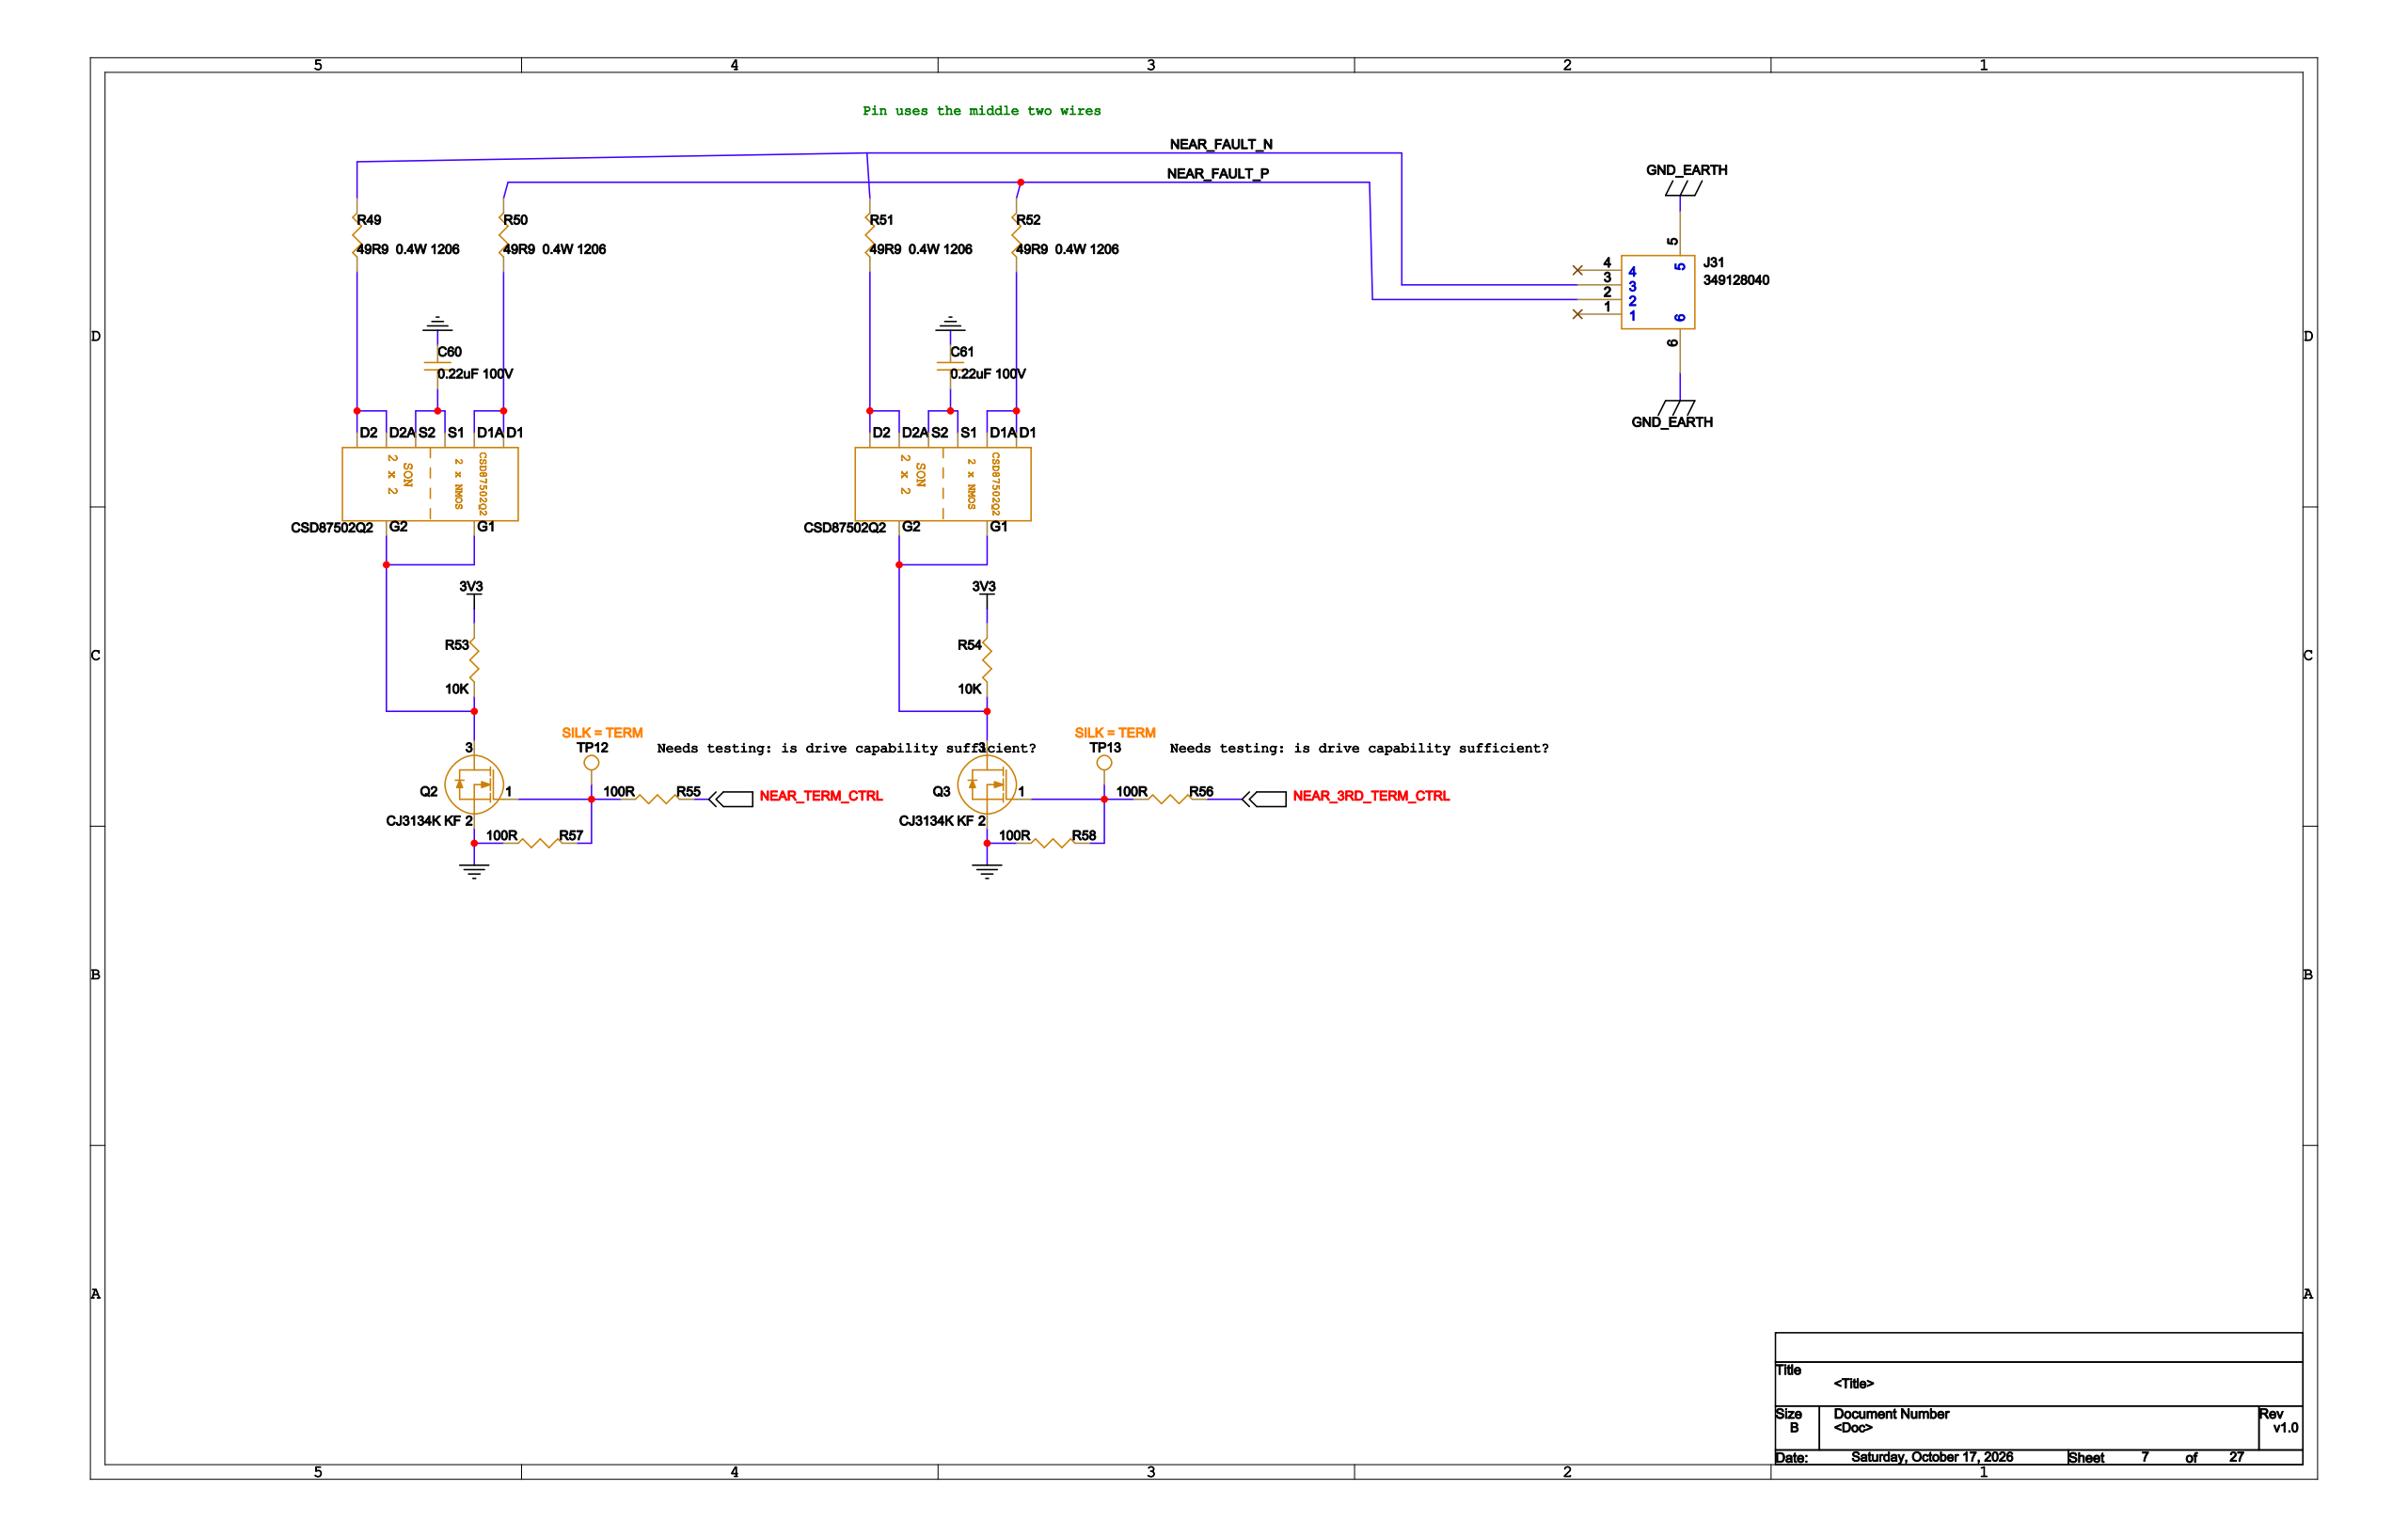Circuit board | Cadence Allegro | 477 parts | 327 nets | one sheet of the schematic
Parts on this sheet (reference | value | footprint):
C60 | 0.22uF 100V | 0805
C61 | 0.22uF 100V | 0805
J31 | 349128040 | 349128040
Q2 | CJ3134K KF | SOT723
Q3 | CJ3134K KF | SOT723
R49 | 49R9  0.4W 1206 | 1206
R50 | 49R9  0.4W 1206 | 1206
R51 | 49R9  0.4W 1206 | 1206
R52 | 49R9  0.4W 1206 | 1206
R53 | 10K | 0402
R54 | 10K | 0402
R55 | 100R | 0402
R56 | 100R | 0402
R57 | 100R | 0402
R58 | 100R | 0402
TP12 | TP | S0400CI
TP13 | TP | S0400CI
Nets of these parts (net: part-pin ...):
GND: C60-1 C61-1 Q2-2 Q3-2 R57-2 R58-2
NEAR_FAULT_N: J31-3 R49-1 R51-1
N16837862: R49-2
NEAR_FAULT_P: J31-2 R50-1 R52-1
N16837864: R50-2
N16837866: R51-2
N16837868: R52-2
3V3: R53-2 R54-2
GND_EARTH: J31-5 J31-6
N16837960: Q2-3 R53-1
N16837964: Q3-3 R54-1
NEAR_3RD_TERM_CTRL: R56-1
NEAR_TERM_CTRL: R55-1
N16837894: C60-2
N16837896: C61-2
N16838062: Q2-1 R55-2 R57-1 TP12-1
N16838077: Q3-1 R56-2 R58-1 TP13-1